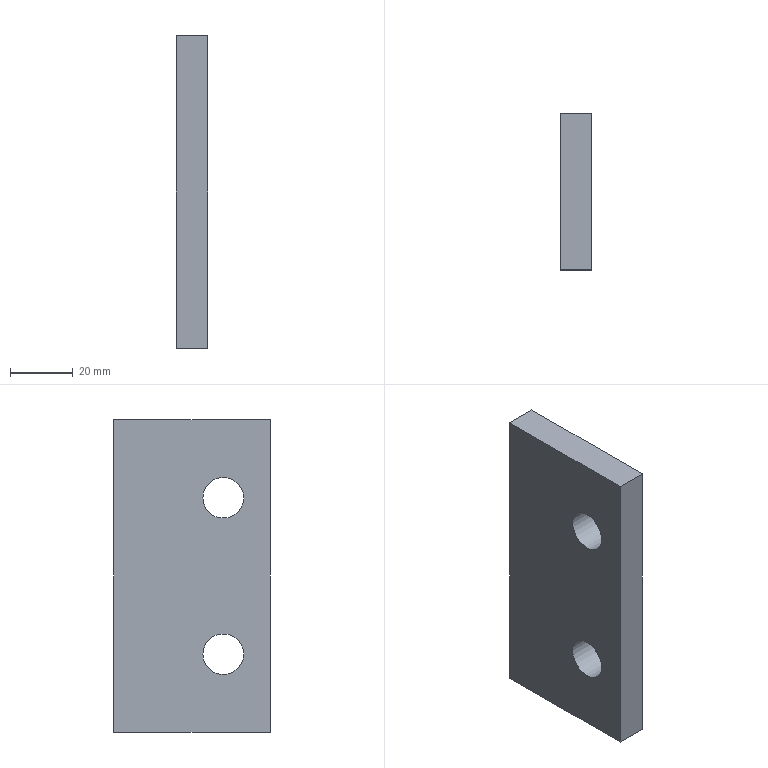Part | NX | features solid 2 | 1 solid | 8 faces | box 10 x 50 x 100 mm | volume 47345 mm3 | plane 6 | cylinder 2 | commonest cylinder face diameters 13 x2
STEP:
#1=CARTESIAN_POINT('',(-1560.,-265.,-502.5));
#2=VERTEX_POINT('',#1);
#3=CARTESIAN_POINT('',(-1560.,-265.,-602.5));
#4=VERTEX_POINT('',#3);
#5=CARTESIAN_POINT('',(-1560.,-265.,-1007.5));
#6=DIRECTION('',(0.,0.,-1.));
#7=VECTOR('',#6,1000.);
#8=LINE('',#5,#7);
#9=EDGE_CURVE('',#2,#4,#8,.T.);
#10=ORIENTED_EDGE('',*,*,#9,.F.);
#11=CARTESIAN_POINT('',(-1550.,-265.,-502.5));
#12=VERTEX_POINT('',#11);
#13=CARTESIAN_POINT('',(-1550.,-265.,-502.5));
#14=DIRECTION('',(-1.,0.,0.));
#15=VECTOR('',#14,1000.);
#16=LINE('',#13,#15);
#17=EDGE_CURVE('',#12,#2,#16,.T.);
#18=ORIENTED_EDGE('',*,*,#17,.F.);
#19=CARTESIAN_POINT('',(-1550.,-265.,-602.5));
#20=VERTEX_POINT('',#19);
#21=CARTESIAN_POINT('',(-1550.,-265.,-1007.5));
#22=DIRECTION('',(0.,0.,-1.));
#23=VECTOR('',#22,1000.);
#24=LINE('',#21,#23);
#25=EDGE_CURVE('',#12,#20,#24,.T.);
#26=ORIENTED_EDGE('',*,*,#25,.T.);
#27=CARTESIAN_POINT('',(-1550.,-265.,-602.5));
#28=DIRECTION('',(-1.,0.,0.));
#29=VECTOR('',#28,1000.);
#30=LINE('',#27,#29);
#31=EDGE_CURVE('',#20,#4,#30,.T.);
#32=ORIENTED_EDGE('',*,*,#31,.T.);
#33=EDGE_LOOP('',(#10,#18,#26,#32));
#34=FACE_BOUND('',#33,.T.);
#35=CARTESIAN_POINT('',(-1550.,-265.,-1007.5));
#36=DIRECTION('',(0.,1.,0.));
#37=DIRECTION('',(-1.,0.,0.));
#38=AXIS2_PLACEMENT_3D('',#35,#36,#37);
#39=PLANE('',#38);
#40=ADVANCED_FACE('',(#34),#39,.T.);
#41=CARTESIAN_POINT('',(-1560.,-315.,-602.5));
#42=VERTEX_POINT('',#41);
#43=CARTESIAN_POINT('',(-1560.,-285.,-602.5));
#44=DIRECTION('',(0.,1.,0.));
#45=VECTOR('',#44,1000.);
#46=LINE('',#43,#45);
#47=EDGE_CURVE('',#42,#4,#46,.T.);
#48=ORIENTED_EDGE('',*,*,#47,.T.);
#49=ORIENTED_EDGE('',*,*,#31,.F.);
#50=CARTESIAN_POINT('',(-1550.,-315.,-602.5));
#51=VERTEX_POINT('',#50);
#52=CARTESIAN_POINT('',(-1550.,-285.,-602.5));
#53=DIRECTION('',(0.,1.,0.));
#54=VECTOR('',#53,1000.);
#55=LINE('',#52,#54);
#56=EDGE_CURVE('',#51,#20,#55,.T.);
#57=ORIENTED_EDGE('',*,*,#56,.F.);
#58=CARTESIAN_POINT('',(-1550.,-315.,-602.5));
#59=DIRECTION('',(-1.,0.,0.));
#60=VECTOR('',#59,1000.);
#61=LINE('',#58,#60);
#62=EDGE_CURVE('',#51,#42,#61,.T.);
#63=ORIENTED_EDGE('',*,*,#62,.T.);
#64=EDGE_LOOP('',(#48,#49,#57,#63));
#65=FACE_BOUND('',#64,.T.);
#66=CARTESIAN_POINT('',(-1550.,-285.,-602.5));
#67=DIRECTION('',(0.,0.,1.));
#68=DIRECTION('',(0.,1.,0.));
#69=AXIS2_PLACEMENT_3D('',#66,#67,#68);
#70=PLANE('',#69);
#71=ADVANCED_FACE('',(#65),#70,.F.);
#72=CARTESIAN_POINT('',(-1560.,-315.,-502.5));
#73=VERTEX_POINT('',#72);
#74=CARTESIAN_POINT('',(-1560.,-315.,-1007.5));
#75=DIRECTION('',(0.,0.,-1.));
#76=VECTOR('',#75,1000.);
#77=LINE('',#74,#76);
#78=EDGE_CURVE('',#73,#42,#77,.T.);
#79=ORIENTED_EDGE('',*,*,#78,.T.);
#80=ORIENTED_EDGE('',*,*,#62,.F.);
#81=CARTESIAN_POINT('',(-1550.,-315.,-502.5));
#82=VERTEX_POINT('',#81);
#83=CARTESIAN_POINT('',(-1550.,-315.,-1007.5));
#84=DIRECTION('',(0.,0.,-1.));
#85=VECTOR('',#84,1000.);
#86=LINE('',#83,#85);
#87=EDGE_CURVE('',#82,#51,#86,.T.);
#88=ORIENTED_EDGE('',*,*,#87,.F.);
#89=CARTESIAN_POINT('',(-1550.,-315.,-502.5));
#90=DIRECTION('',(-1.,0.,0.));
#91=VECTOR('',#90,1000.);
#92=LINE('',#89,#91);
#93=EDGE_CURVE('',#82,#73,#92,.T.);
#94=ORIENTED_EDGE('',*,*,#93,.T.);
#95=EDGE_LOOP('',(#79,#80,#88,#94));
#96=FACE_BOUND('',#95,.T.);
#97=CARTESIAN_POINT('',(-1550.,-315.,-1007.5));
#98=DIRECTION('',(0.,1.,0.));
#99=DIRECTION('',(-1.,0.,0.));
#100=AXIS2_PLACEMENT_3D('',#97,#98,#99);
#101=PLANE('',#100);
#102=ADVANCED_FACE('',(#96),#101,.F.);
#103=CARTESIAN_POINT('',(-1550.,-293.5,-527.5));
#104=VERTEX_POINT('',#103);
#105=CARTESIAN_POINT('',(-1550.,-300.,-527.5));
#106=DIRECTION('',(1.,0.,0.));
#107=DIRECTION('',(0.,1.,0.));
#108=AXIS2_PLACEMENT_3D('',#105,#106,#107);
#109=CIRCLE('',#108,6.5);
#110=EDGE_CURVE('',#104,#104,#109,.T.);
#111=ORIENTED_EDGE('',*,*,#110,.T.);
#112=EDGE_LOOP('',(#111));
#113=FACE_BOUND('',#112,.T.);
#114=CARTESIAN_POINT('',(-1560.,-293.5,-527.5));
#115=VERTEX_POINT('',#114);
#116=CARTESIAN_POINT('',(-1560.,-300.,-527.5));
#117=DIRECTION('',(1.,0.,0.));
#118=DIRECTION('',(0.,1.,0.));
#119=AXIS2_PLACEMENT_3D('',#116,#117,#118);
#120=CIRCLE('',#119,6.5);
#121=EDGE_CURVE('',#115,#115,#120,.T.);
#122=ORIENTED_EDGE('',*,*,#121,.F.);
#123=EDGE_LOOP('',(#122));
#124=FACE_BOUND('',#123,.T.);
#125=CARTESIAN_POINT('',(-1550.,-300.,-527.5));
#126=DIRECTION('',(-1.,0.,0.));
#127=DIRECTION('',(0.,-1.,0.));
#128=AXIS2_PLACEMENT_3D('',#125,#126,#127);
#129=CYLINDRICAL_SURFACE('',#128,6.5);
#130=ADVANCED_FACE('',(#113,#124),#129,.F.);
#131=CARTESIAN_POINT('',(-1550.,-293.5,-577.5));
#132=VERTEX_POINT('',#131);
#133=CARTESIAN_POINT('',(-1550.,-300.,-577.5));
#134=DIRECTION('',(1.,0.,0.));
#135=DIRECTION('',(0.,1.,0.));
#136=AXIS2_PLACEMENT_3D('',#133,#134,#135);
#137=CIRCLE('',#136,6.5);
#138=EDGE_CURVE('',#132,#132,#137,.T.);
#139=ORIENTED_EDGE('',*,*,#138,.T.);
#140=EDGE_LOOP('',(#139));
#141=FACE_BOUND('',#140,.T.);
#142=CARTESIAN_POINT('',(-1560.,-293.5,-577.5));
#143=VERTEX_POINT('',#142);
#144=CARTESIAN_POINT('',(-1560.,-300.,-577.5));
#145=DIRECTION('',(1.,0.,0.));
#146=DIRECTION('',(0.,1.,0.));
#147=AXIS2_PLACEMENT_3D('',#144,#145,#146);
#148=CIRCLE('',#147,6.5);
#149=EDGE_CURVE('',#143,#143,#148,.T.);
#150=ORIENTED_EDGE('',*,*,#149,.F.);
#151=EDGE_LOOP('',(#150));
#152=FACE_BOUND('',#151,.T.);
#153=CARTESIAN_POINT('',(-1550.,-300.,-577.5));
#154=DIRECTION('',(-1.,0.,0.));
#155=DIRECTION('',(0.,-1.,0.));
#156=AXIS2_PLACEMENT_3D('',#153,#154,#155);
#157=CYLINDRICAL_SURFACE('',#156,6.5);
#158=ADVANCED_FACE('',(#141,#152),#157,.F.);
#159=CARTESIAN_POINT('',(-1560.,-285.,-502.5));
#160=DIRECTION('',(0.,1.,0.));
#161=VECTOR('',#160,1000.);
#162=LINE('',#159,#161);
#163=EDGE_CURVE('',#73,#2,#162,.T.);
#164=ORIENTED_EDGE('',*,*,#163,.F.);
#165=ORIENTED_EDGE('',*,*,#93,.F.);
#166=CARTESIAN_POINT('',(-1550.,-285.,-502.5));
#167=DIRECTION('',(0.,1.,0.));
#168=VECTOR('',#167,1000.);
#169=LINE('',#166,#168);
#170=EDGE_CURVE('',#82,#12,#169,.T.);
#171=ORIENTED_EDGE('',*,*,#170,.T.);
#172=ORIENTED_EDGE('',*,*,#17,.T.);
#173=EDGE_LOOP('',(#164,#165,#171,#172));
#174=FACE_BOUND('',#173,.T.);
#175=CARTESIAN_POINT('',(-1550.,-285.,-502.5));
#176=DIRECTION('',(0.,0.,1.));
#177=DIRECTION('',(0.,1.,0.));
#178=AXIS2_PLACEMENT_3D('',#175,#176,#177);
#179=PLANE('',#178);
#180=ADVANCED_FACE('',(#174),#179,.T.);
#181=ORIENTED_EDGE('',*,*,#138,.F.);
#182=EDGE_LOOP('',(#181));
#183=FACE_BOUND('',#182,.T.);
#184=ORIENTED_EDGE('',*,*,#110,.F.);
#185=EDGE_LOOP('',(#184));
#186=FACE_BOUND('',#185,.T.);
#187=ORIENTED_EDGE('',*,*,#25,.F.);
#188=ORIENTED_EDGE('',*,*,#170,.F.);
#189=ORIENTED_EDGE('',*,*,#87,.T.);
#190=ORIENTED_EDGE('',*,*,#56,.T.);
#191=EDGE_LOOP('',(#187,#188,#189,#190));
#192=FACE_BOUND('',#191,.T.);
#193=CARTESIAN_POINT('',(-1550.,-285.,-1007.5));
#194=DIRECTION('',(1.,0.,0.));
#195=DIRECTION('',(0.,1.,0.));
#196=AXIS2_PLACEMENT_3D('',#193,#194,#195);
#197=PLANE('',#196);
#198=ADVANCED_FACE('',(#183,#186,#192),#197,.T.);
#199=ORIENTED_EDGE('',*,*,#149,.T.);
#200=EDGE_LOOP('',(#199));
#201=FACE_BOUND('',#200,.T.);
#202=ORIENTED_EDGE('',*,*,#121,.T.);
#203=EDGE_LOOP('',(#202));
#204=FACE_BOUND('',#203,.T.);
#205=ORIENTED_EDGE('',*,*,#9,.T.);
#206=ORIENTED_EDGE('',*,*,#47,.F.);
#207=ORIENTED_EDGE('',*,*,#78,.F.);
#208=ORIENTED_EDGE('',*,*,#163,.T.);
#209=EDGE_LOOP('',(#205,#206,#207,#208));
#210=FACE_BOUND('',#209,.T.);
#211=CARTESIAN_POINT('',(-1560.,-285.,-1007.5));
#212=DIRECTION('',(1.,0.,0.));
#213=DIRECTION('',(0.,1.,0.));
#214=AXIS2_PLACEMENT_3D('',#211,#212,#213);
#215=PLANE('',#214);
#216=ADVANCED_FACE('',(#201,#204,#210),#215,.F.);
#217=CLOSED_SHELL('',(#40,#71,#102,#130,#158,#180,#198,#216));
#218=MANIFOLD_SOLID_BREP('',#217);
#219=(LENGTH_UNIT()NAMED_UNIT(*)SI_UNIT(.MILLI.,.METRE.));
#220=UNCERTAINTY_MEASURE_WITH_UNIT(LENGTH_MEASURE(0.00001),#219,'','');
#221=(NAMED_UNIT(*)PLANE_ANGLE_UNIT()SI_UNIT($,.RADIAN.));
#222=(NAMED_UNIT(*)SI_UNIT($,.STERADIAN.)SOLID_ANGLE_UNIT());
#223=(GEOMETRIC_REPRESENTATION_CONTEXT(3)GLOBAL_UNCERTAINTY_ASSIGNED_CONTEXT((#220))GLOBAL_UNIT_ASSIGNED_CONTEXT((#219,#221,#222))REPRESENTATION_CONTEXT('',''));
#224=ADVANCED_BREP_SHAPE_REPRESENTATION('',(#218),#223);